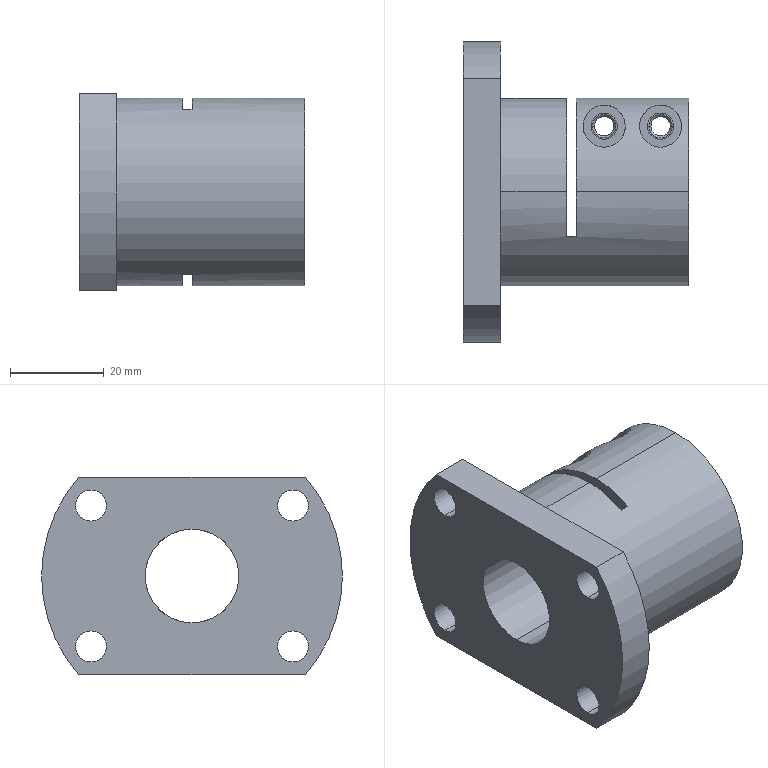Part | STEP file | 11-STHWCBL20byizai20060711 | 1 solid | 50 faces | box 48 x 64 x 42 mm | volume 50580 mm3 | cylinder 30 | plane 14 | cone 6 | commonest cylinder face diameters 6.6 x8 4.134 x4 5.6 x4 9 x4 20 x4 40 x4